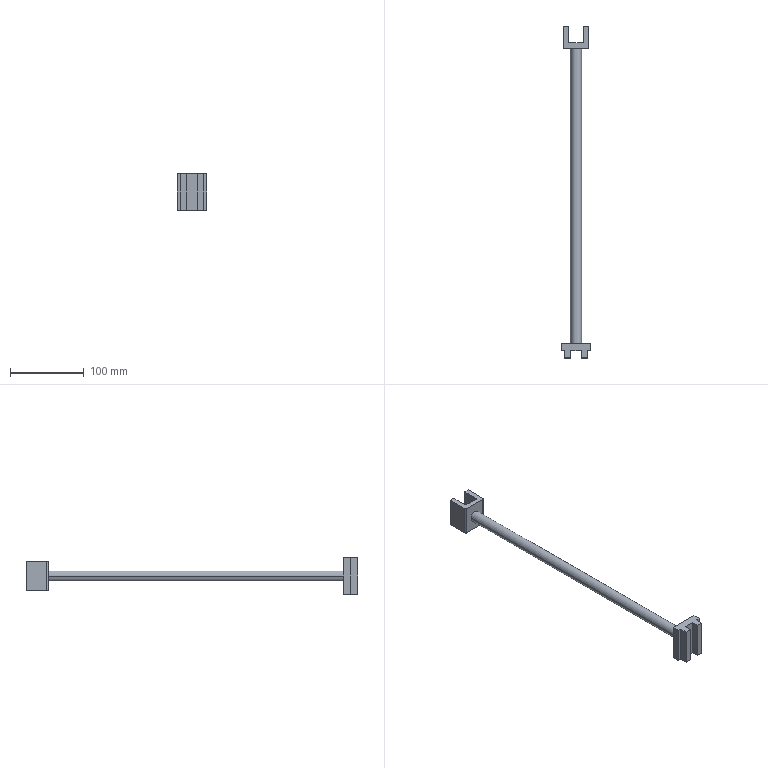Part | SolidWorks | features ICE 3, Extrusion 1, Fillet 1 | 1 solid | 30 faces | box 40 x 450 x 50 mm | volume 121566 mm3 | plane 24 | cylinder 6 | commonest cylinder face diameters 4 x4 15 x2
STEP:
#1=CARTESIAN_POINT('',(7.5,-415.,0.));
#2=VERTEX_POINT('',#1);
#3=CARTESIAN_POINT('',(-7.5,-415.,0.));
#4=VERTEX_POINT('',#3);
#5=CARTESIAN_POINT('',(0.,-415.,0.));
#6=DIRECTION('',(0.,-1.,0.));
#7=DIRECTION('',(1.,0.,0.));
#8=AXIS2_PLACEMENT_3D('',#5,#6,#7);
#9=CIRCLE('',#8,7.5);
#10=EDGE_CURVE('',#2,#4,#9,.T.);
#11=ORIENTED_EDGE('',*,*,#10,.F.);
#12=CARTESIAN_POINT('',(7.5,-15.,0.));
#13=VERTEX_POINT('',#12);
#14=CARTESIAN_POINT('',(7.5,-415.,0.));
#15=DIRECTION('',(0.,1.,0.));
#16=VECTOR('',#15,1000.);
#17=LINE('',#14,#16);
#18=EDGE_CURVE('',#2,#13,#17,.T.);
#19=ORIENTED_EDGE('',*,*,#18,.T.);
#20=CARTESIAN_POINT('',(-7.5,-15.,0.));
#21=VERTEX_POINT('',#20);
#22=CARTESIAN_POINT('',(0.,-15.,0.));
#23=DIRECTION('',(0.,-1.,0.));
#24=DIRECTION('',(-1.,0.,0.));
#25=AXIS2_PLACEMENT_3D('',#22,#23,#24);
#26=CIRCLE('',#25,7.5);
#27=EDGE_CURVE('',#13,#21,#26,.T.);
#28=ORIENTED_EDGE('',*,*,#27,.T.);
#29=CARTESIAN_POINT('',(-7.5,-415.,0.));
#30=DIRECTION('',(0.,1.,0.));
#31=VECTOR('',#30,1000.);
#32=LINE('',#29,#31);
#33=EDGE_CURVE('',#4,#21,#32,.T.);
#34=ORIENTED_EDGE('',*,*,#33,.F.);
#35=EDGE_LOOP('',(#11,#19,#28,#34));
#36=FACE_OUTER_BOUND('',#35,.T.);
#37=CARTESIAN_POINT('',(0.,-415.,0.));
#38=DIRECTION('',(0.,1.,0.));
#39=DIRECTION('',(-1.,0.,0.));
#40=AXIS2_PLACEMENT_3D('',#37,#38,#39);
#41=CYLINDRICAL_SURFACE('',#40,7.5);
#42=ADVANCED_FACE('',(#36),#41,.T.);
#43=CARTESIAN_POINT('',(20.,-425.,25.));
#44=VERTEX_POINT('',#43);
#45=CARTESIAN_POINT('',(15.1,-425.,25.));
#46=VERTEX_POINT('',#45);
#47=CARTESIAN_POINT('',(-20.,-425.,25.));
#48=DIRECTION('',(-1.,0.,0.));
#49=VECTOR('',#48,1000.);
#50=LINE('',#47,#49);
#51=EDGE_CURVE('',#44,#46,#50,.T.);
#52=ORIENTED_EDGE('',*,*,#51,.T.);
#53=CARTESIAN_POINT('',(15.1,-425.,-25.));
#54=VERTEX_POINT('',#53);
#55=CARTESIAN_POINT('',(15.1,-425.,25.));
#56=DIRECTION('',(0.,0.,1.));
#57=VECTOR('',#56,1000.);
#58=LINE('',#55,#57);
#59=EDGE_CURVE('',#54,#46,#58,.T.);
#60=ORIENTED_EDGE('',*,*,#59,.F.);
#61=CARTESIAN_POINT('',(20.,-425.,-25.));
#62=VERTEX_POINT('',#61);
#63=CARTESIAN_POINT('',(-20.,-425.,-25.));
#64=DIRECTION('',(1.,0.,0.));
#65=VECTOR('',#64,1000.);
#66=LINE('',#63,#65);
#67=EDGE_CURVE('',#54,#62,#66,.T.);
#68=ORIENTED_EDGE('',*,*,#67,.T.);
#69=CARTESIAN_POINT('',(20.,-425.,25.));
#70=DIRECTION('',(0.,0.,1.));
#71=VECTOR('',#70,1000.);
#72=LINE('',#69,#71);
#73=EDGE_CURVE('',#62,#44,#72,.T.);
#74=ORIENTED_EDGE('',*,*,#73,.T.);
#75=EDGE_LOOP('',(#52,#60,#68,#74));
#76=FACE_OUTER_BOUND('',#75,.T.);
#77=CARTESIAN_POINT('',(0.,-425.,0.));
#78=DIRECTION('',(0.,-1.,0.));
#79=DIRECTION('',(0.,0.,-1.));
#80=AXIS2_PLACEMENT_3D('',#77,#78,#79);
#81=PLANE('',#80);
#82=ADVANCED_FACE('',(#76),#81,.T.);
#83=CARTESIAN_POINT('',(-6.9,-425.,-25.));
#84=VERTEX_POINT('',#83);
#85=CARTESIAN_POINT('',(6.9,-425.,-25.));
#86=VERTEX_POINT('',#85);
#87=CARTESIAN_POINT('',(-20.,-425.,-25.));
#88=DIRECTION('',(1.,0.,0.));
#89=VECTOR('',#88,1000.);
#90=LINE('',#87,#89);
#91=EDGE_CURVE('',#84,#86,#90,.T.);
#92=ORIENTED_EDGE('',*,*,#91,.T.);
#93=CARTESIAN_POINT('',(6.9,-425.,25.));
#94=VERTEX_POINT('',#93);
#95=CARTESIAN_POINT('',(6.9,-425.,25.));
#96=DIRECTION('',(0.,0.,-1.));
#97=VECTOR('',#96,1000.);
#98=LINE('',#95,#97);
#99=EDGE_CURVE('',#94,#86,#98,.T.);
#100=ORIENTED_EDGE('',*,*,#99,.F.);
#101=CARTESIAN_POINT('',(-6.9,-425.,25.));
#102=VERTEX_POINT('',#101);
#103=CARTESIAN_POINT('',(-20.,-425.,25.));
#104=DIRECTION('',(-1.,0.,0.));
#105=VECTOR('',#104,1000.);
#106=LINE('',#103,#105);
#107=EDGE_CURVE('',#94,#102,#106,.T.);
#108=ORIENTED_EDGE('',*,*,#107,.T.);
#109=CARTESIAN_POINT('',(-6.9,-425.,25.));
#110=DIRECTION('',(0.,0.,1.));
#111=VECTOR('',#110,1000.);
#112=LINE('',#109,#111);
#113=EDGE_CURVE('',#84,#102,#112,.T.);
#114=ORIENTED_EDGE('',*,*,#113,.F.);
#115=EDGE_LOOP('',(#92,#100,#108,#114));
#116=FACE_OUTER_BOUND('',#115,.T.);
#117=CARTESIAN_POINT('',(0.,-425.,0.));
#118=DIRECTION('',(0.,-1.,0.));
#119=DIRECTION('',(0.,0.,-1.));
#120=AXIS2_PLACEMENT_3D('',#117,#118,#119);
#121=PLANE('',#120);
#122=ADVANCED_FACE('',(#116),#121,.T.);
#123=CARTESIAN_POINT('',(17.5,-13.,20.));
#124=VERTEX_POINT('',#123);
#125=CARTESIAN_POINT('',(17.5,15.,20.));
#126=VERTEX_POINT('',#125);
#127=CARTESIAN_POINT('',(17.5,15.,20.));
#128=DIRECTION('',(0.,1.,0.));
#129=VECTOR('',#128,1000.);
#130=LINE('',#127,#129);
#131=EDGE_CURVE('',#124,#126,#130,.T.);
#132=ORIENTED_EDGE('',*,*,#131,.F.);
#133=CARTESIAN_POINT('',(17.5,-13.,-20.));
#134=VERTEX_POINT('',#133);
#135=CARTESIAN_POINT('',(17.5,-13.,20.));
#136=DIRECTION('',(0.,0.,-1.));
#137=VECTOR('',#136,1000.);
#138=LINE('',#135,#137);
#139=EDGE_CURVE('',#124,#134,#138,.T.);
#140=ORIENTED_EDGE('',*,*,#139,.T.);
#141=CARTESIAN_POINT('',(17.5,15.,-20.));
#142=VERTEX_POINT('',#141);
#143=CARTESIAN_POINT('',(17.5,15.,-20.));
#144=DIRECTION('',(0.,1.,0.));
#145=VECTOR('',#144,1000.);
#146=LINE('',#143,#145);
#147=EDGE_CURVE('',#134,#142,#146,.T.);
#148=ORIENTED_EDGE('',*,*,#147,.T.);
#149=CARTESIAN_POINT('',(17.5,15.,20.));
#150=DIRECTION('',(0.,0.,-1.));
#151=VECTOR('',#150,1000.);
#152=LINE('',#149,#151);
#153=EDGE_CURVE('',#126,#142,#152,.T.);
#154=ORIENTED_EDGE('',*,*,#153,.F.);
#155=EDGE_LOOP('',(#132,#140,#148,#154));
#156=FACE_OUTER_BOUND('',#155,.T.);
#157=CARTESIAN_POINT('',(17.5,15.,20.));
#158=DIRECTION('',(-1.,0.,0.));
#159=DIRECTION('',(0.,-1.,0.));
#160=AXIS2_PLACEMENT_3D('',#157,#158,#159);
#161=PLANE('',#160);
#162=ADVANCED_FACE('',(#156),#161,.F.);
#163=CARTESIAN_POINT('',(10.5,15.,-20.));
#164=VERTEX_POINT('',#163);
#165=CARTESIAN_POINT('',(10.5,15.,-20.));
#166=DIRECTION('',(-1.,0.,0.));
#167=VECTOR('',#166,1000.);
#168=LINE('',#165,#167);
#169=EDGE_CURVE('',#142,#164,#168,.T.);
#170=ORIENTED_EDGE('',*,*,#169,.T.);
#171=CARTESIAN_POINT('',(10.5,15.,20.));
#172=VERTEX_POINT('',#171);
#173=CARTESIAN_POINT('',(10.5,15.,20.));
#174=DIRECTION('',(0.,0.,-1.));
#175=VECTOR('',#174,1000.);
#176=LINE('',#173,#175);
#177=EDGE_CURVE('',#172,#164,#176,.T.);
#178=ORIENTED_EDGE('',*,*,#177,.F.);
#179=CARTESIAN_POINT('',(10.5,15.,20.));
#180=DIRECTION('',(-1.,0.,0.));
#181=VECTOR('',#180,1000.);
#182=LINE('',#179,#181);
#183=EDGE_CURVE('',#126,#172,#182,.T.);
#184=ORIENTED_EDGE('',*,*,#183,.F.);
#185=ORIENTED_EDGE('',*,*,#153,.T.);
#186=EDGE_LOOP('',(#170,#178,#184,#185));
#187=FACE_OUTER_BOUND('',#186,.T.);
#188=CARTESIAN_POINT('',(10.5,15.,20.));
#189=DIRECTION('',(0.,-1.,0.));
#190=DIRECTION('',(0.,0.,-1.));
#191=AXIS2_PLACEMENT_3D('',#188,#189,#190);
#192=PLANE('',#191);
#193=ADVANCED_FACE('',(#187),#192,.F.);
#194=CARTESIAN_POINT('',(10.5,-6.,-20.));
#195=VERTEX_POINT('',#194);
#196=CARTESIAN_POINT('',(10.5,8.,-20.));
#197=DIRECTION('',(0.,-1.,0.));
#198=VECTOR('',#197,1000.);
#199=LINE('',#196,#198);
#200=EDGE_CURVE('',#164,#195,#199,.T.);
#201=ORIENTED_EDGE('',*,*,#200,.T.);
#202=CARTESIAN_POINT('',(10.5,-6.,20.));
#203=VERTEX_POINT('',#202);
#204=CARTESIAN_POINT('',(10.5,-6.,20.));
#205=DIRECTION('',(0.,0.,1.));
#206=VECTOR('',#205,1000.);
#207=LINE('',#204,#206);
#208=EDGE_CURVE('',#195,#203,#207,.T.);
#209=ORIENTED_EDGE('',*,*,#208,.T.);
#210=CARTESIAN_POINT('',(10.5,8.,20.));
#211=DIRECTION('',(0.,-1.,0.));
#212=VECTOR('',#211,1000.);
#213=LINE('',#210,#212);
#214=EDGE_CURVE('',#172,#203,#213,.T.);
#215=ORIENTED_EDGE('',*,*,#214,.F.);
#216=ORIENTED_EDGE('',*,*,#177,.T.);
#217=EDGE_LOOP('',(#201,#209,#215,#216));
#218=FACE_OUTER_BOUND('',#217,.T.);
#219=CARTESIAN_POINT('',(10.5,8.,20.));
#220=DIRECTION('',(1.,0.,0.));
#221=DIRECTION('',(0.,1.,0.));
#222=AXIS2_PLACEMENT_3D('',#219,#220,#221);
#223=PLANE('',#222);
#224=ADVANCED_FACE('',(#218),#223,.F.);
#225=CARTESIAN_POINT('',(8.5,-8.,20.));
#226=VERTEX_POINT('',#225);
#227=CARTESIAN_POINT('',(-8.5,-8.,20.));
#228=VERTEX_POINT('',#227);
#229=CARTESIAN_POINT('',(-10.5,-8.,20.));
#230=DIRECTION('',(-1.,0.,0.));
#231=VECTOR('',#230,1000.);
#232=LINE('',#229,#231);
#233=EDGE_CURVE('',#226,#228,#232,.T.);
#234=ORIENTED_EDGE('',*,*,#233,.F.);
#235=CARTESIAN_POINT('',(8.5,-8.,-20.));
#236=VERTEX_POINT('',#235);
#237=CARTESIAN_POINT('',(8.5,-8.,-20.));
#238=DIRECTION('',(0.,0.,-1.));
#239=VECTOR('',#238,1000.);
#240=LINE('',#237,#239);
#241=EDGE_CURVE('',#226,#236,#240,.T.);
#242=ORIENTED_EDGE('',*,*,#241,.T.);
#243=CARTESIAN_POINT('',(-8.5,-8.,-20.));
#244=VERTEX_POINT('',#243);
#245=CARTESIAN_POINT('',(-10.5,-8.,-20.));
#246=DIRECTION('',(-1.,0.,0.));
#247=VECTOR('',#246,1000.);
#248=LINE('',#245,#247);
#249=EDGE_CURVE('',#236,#244,#248,.T.);
#250=ORIENTED_EDGE('',*,*,#249,.T.);
#251=CARTESIAN_POINT('',(-8.5,-8.,20.));
#252=DIRECTION('',(0.,0.,1.));
#253=VECTOR('',#252,1000.);
#254=LINE('',#251,#253);
#255=EDGE_CURVE('',#244,#228,#254,.T.);
#256=ORIENTED_EDGE('',*,*,#255,.T.);
#257=EDGE_LOOP('',(#234,#242,#250,#256));
#258=FACE_OUTER_BOUND('',#257,.T.);
#259=CARTESIAN_POINT('',(-10.5,-8.,20.));
#260=DIRECTION('',(0.,-1.,0.));
#261=DIRECTION('',(0.,0.,-1.));
#262=AXIS2_PLACEMENT_3D('',#259,#260,#261);
#263=PLANE('',#262);
#264=ADVANCED_FACE('',(#258),#263,.F.);
#265=CARTESIAN_POINT('',(-10.5,-6.,20.));
#266=VERTEX_POINT('',#265);
#267=CARTESIAN_POINT('',(-10.5,15.,20.));
#268=VERTEX_POINT('',#267);
#269=CARTESIAN_POINT('',(-10.5,8.,20.));
#270=DIRECTION('',(0.,1.,0.));
#271=VECTOR('',#270,1000.);
#272=LINE('',#269,#271);
#273=EDGE_CURVE('',#266,#268,#272,.T.);
#274=ORIENTED_EDGE('',*,*,#273,.F.);
#275=CARTESIAN_POINT('',(-10.5,-6.,-20.));
#276=VERTEX_POINT('',#275);
#277=CARTESIAN_POINT('',(-10.5,-6.,-20.));
#278=DIRECTION('',(0.,0.,-1.));
#279=VECTOR('',#278,1000.);
#280=LINE('',#277,#279);
#281=EDGE_CURVE('',#266,#276,#280,.T.);
#282=ORIENTED_EDGE('',*,*,#281,.T.);
#283=CARTESIAN_POINT('',(-10.5,15.,-20.));
#284=VERTEX_POINT('',#283);
#285=CARTESIAN_POINT('',(-10.5,8.,-20.));
#286=DIRECTION('',(0.,1.,0.));
#287=VECTOR('',#286,1000.);
#288=LINE('',#285,#287);
#289=EDGE_CURVE('',#276,#284,#288,.T.);
#290=ORIENTED_EDGE('',*,*,#289,.T.);
#291=CARTESIAN_POINT('',(-10.5,15.,20.));
#292=DIRECTION('',(0.,0.,-1.));
#293=VECTOR('',#292,1000.);
#294=LINE('',#291,#293);
#295=EDGE_CURVE('',#268,#284,#294,.T.);
#296=ORIENTED_EDGE('',*,*,#295,.F.);
#297=EDGE_LOOP('',(#274,#282,#290,#296));
#298=FACE_OUTER_BOUND('',#297,.T.);
#299=CARTESIAN_POINT('',(-10.5,8.,20.));
#300=DIRECTION('',(-1.,0.,0.));
#301=DIRECTION('',(0.,-1.,0.));
#302=AXIS2_PLACEMENT_3D('',#299,#300,#301);
#303=PLANE('',#302);
#304=ADVANCED_FACE('',(#298),#303,.F.);
#305=CARTESIAN_POINT('',(-17.5,15.,-20.));
#306=VERTEX_POINT('',#305);
#307=CARTESIAN_POINT('',(-17.5,15.,-20.));
#308=DIRECTION('',(-1.,0.,0.));
#309=VECTOR('',#308,1000.);
#310=LINE('',#307,#309);
#311=EDGE_CURVE('',#284,#306,#310,.T.);
#312=ORIENTED_EDGE('',*,*,#311,.T.);
#313=CARTESIAN_POINT('',(-17.5,15.,20.));
#314=VERTEX_POINT('',#313);
#315=CARTESIAN_POINT('',(-17.5,15.,20.));
#316=DIRECTION('',(0.,0.,-1.));
#317=VECTOR('',#316,1000.);
#318=LINE('',#315,#317);
#319=EDGE_CURVE('',#314,#306,#318,.T.);
#320=ORIENTED_EDGE('',*,*,#319,.F.);
#321=CARTESIAN_POINT('',(-17.5,15.,20.));
#322=DIRECTION('',(-1.,0.,0.));
#323=VECTOR('',#322,1000.);
#324=LINE('',#321,#323);
#325=EDGE_CURVE('',#268,#314,#324,.T.);
#326=ORIENTED_EDGE('',*,*,#325,.F.);
#327=ORIENTED_EDGE('',*,*,#295,.T.);
#328=EDGE_LOOP('',(#312,#320,#326,#327));
#329=FACE_OUTER_BOUND('',#328,.T.);
#330=CARTESIAN_POINT('',(-17.5,15.,20.));
#331=DIRECTION('',(0.,-1.,0.));
#332=DIRECTION('',(0.,0.,-1.));
#333=AXIS2_PLACEMENT_3D('',#330,#331,#332);
#334=PLANE('',#333);
#335=ADVANCED_FACE('',(#329),#334,.F.);
#336=CARTESIAN_POINT('',(-17.5,-13.,-20.));
#337=VERTEX_POINT('',#336);
#338=CARTESIAN_POINT('',(-17.5,15.,-20.));
#339=DIRECTION('',(0.,-1.,0.));
#340=VECTOR('',#339,1000.);
#341=LINE('',#338,#340);
#342=EDGE_CURVE('',#306,#337,#341,.T.);
#343=ORIENTED_EDGE('',*,*,#342,.T.);
#344=CARTESIAN_POINT('',(-17.5,-13.,20.));
#345=VERTEX_POINT('',#344);
#346=CARTESIAN_POINT('',(-17.5,-13.,20.));
#347=DIRECTION('',(0.,0.,1.));
#348=VECTOR('',#347,1000.);
#349=LINE('',#346,#348);
#350=EDGE_CURVE('',#337,#345,#349,.T.);
#351=ORIENTED_EDGE('',*,*,#350,.T.);
#352=CARTESIAN_POINT('',(-17.5,15.,20.));
#353=DIRECTION('',(0.,-1.,0.));
#354=VECTOR('',#353,1000.);
#355=LINE('',#352,#354);
#356=EDGE_CURVE('',#314,#345,#355,.T.);
#357=ORIENTED_EDGE('',*,*,#356,.F.);
#358=ORIENTED_EDGE('',*,*,#319,.T.);
#359=EDGE_LOOP('',(#343,#351,#357,#358));
#360=FACE_OUTER_BOUND('',#359,.T.);
#361=CARTESIAN_POINT('',(-17.5,15.,20.));
#362=DIRECTION('',(1.,0.,0.));
#363=DIRECTION('',(0.,1.,0.));
#364=AXIS2_PLACEMENT_3D('',#361,#362,#363);
#365=PLANE('',#364);
#366=ADVANCED_FACE('',(#360),#365,.F.);
#367=CARTESIAN_POINT('',(0.,-15.,0.));
#368=DIRECTION('',(0.,-1.,0.));
#369=DIRECTION('',(-1.,0.,0.));
#370=AXIS2_PLACEMENT_3D('',#367,#368,#369);
#371=CIRCLE('',#370,7.5);
#372=EDGE_CURVE('',#21,#13,#371,.T.);
#373=ORIENTED_EDGE('',*,*,#372,.F.);
#374=ORIENTED_EDGE('',*,*,#27,.F.);
#375=EDGE_LOOP('',(#373,#374));
#376=FACE_BOUND('',#375,.T.);
#377=CARTESIAN_POINT('',(-15.5,-15.,-20.));
#378=VERTEX_POINT('',#377);
#379=CARTESIAN_POINT('',(15.5,-15.,-20.));
#380=VERTEX_POINT('',#379);
#381=CARTESIAN_POINT('',(-17.5,-15.,-20.));
#382=DIRECTION('',(1.,0.,0.));
#383=VECTOR('',#382,1000.);
#384=LINE('',#381,#383);
#385=EDGE_CURVE('',#378,#380,#384,.T.);
#386=ORIENTED_EDGE('',*,*,#385,.T.);
#387=CARTESIAN_POINT('',(15.5,-15.,20.));
#388=VERTEX_POINT('',#387);
#389=CARTESIAN_POINT('',(15.5,-15.,20.));
#390=DIRECTION('',(0.,0.,1.));
#391=VECTOR('',#390,1000.);
#392=LINE('',#389,#391);
#393=EDGE_CURVE('',#380,#388,#392,.T.);
#394=ORIENTED_EDGE('',*,*,#393,.T.);
#395=CARTESIAN_POINT('',(-15.5,-15.,20.));
#396=VERTEX_POINT('',#395);
#397=CARTESIAN_POINT('',(-17.5,-15.,20.));
#398=DIRECTION('',(1.,0.,0.));
#399=VECTOR('',#398,1000.);
#400=LINE('',#397,#399);
#401=EDGE_CURVE('',#396,#388,#400,.T.);
#402=ORIENTED_EDGE('',*,*,#401,.F.);
#403=CARTESIAN_POINT('',(-15.5,-15.,20.));
#404=DIRECTION('',(0.,0.,-1.));
#405=VECTOR('',#404,1000.);
#406=LINE('',#403,#405);
#407=EDGE_CURVE('',#396,#378,#406,.T.);
#408=ORIENTED_EDGE('',*,*,#407,.T.);
#409=EDGE_LOOP('',(#386,#394,#402,#408));
#410=FACE_OUTER_BOUND('',#409,.T.);
#411=CARTESIAN_POINT('',(-17.5,-15.,20.));
#412=DIRECTION('',(0.,1.,0.));
#413=DIRECTION('',(-1.,0.,0.));
#414=AXIS2_PLACEMENT_3D('',#411,#412,#413);
#415=PLANE('',#414);
#416=ADVANCED_FACE('',(#376,#410),#415,.F.);
#417=ORIENTED_EDGE('',*,*,#401,.T.);
#418=CARTESIAN_POINT('',(15.5,-13.,20.));
#419=DIRECTION('',(0.,0.,1.));
#420=DIRECTION('',(1.,0.,0.));
#421=AXIS2_PLACEMENT_3D('',#418,#419,#420);
#422=CIRCLE('',#421,2.);
#423=EDGE_CURVE('',#388,#124,#422,.T.);
#424=ORIENTED_EDGE('',*,*,#423,.T.);
#425=ORIENTED_EDGE('',*,*,#131,.T.);
#426=ORIENTED_EDGE('',*,*,#183,.T.);
#427=ORIENTED_EDGE('',*,*,#214,.T.);
#428=CARTESIAN_POINT('',(8.5,-6.,20.));
#429=DIRECTION('',(0.,0.,-1.));
#430=DIRECTION('',(1.,0.,0.));
#431=AXIS2_PLACEMENT_3D('',#428,#429,#430);
#432=CIRCLE('',#431,2.);
#433=EDGE_CURVE('',#203,#226,#432,.T.);
#434=ORIENTED_EDGE('',*,*,#433,.T.);
#435=ORIENTED_EDGE('',*,*,#233,.T.);
#436=CARTESIAN_POINT('',(-8.5,-6.,20.));
#437=DIRECTION('',(0.,0.,-1.));
#438=DIRECTION('',(1.,0.,0.));
#439=AXIS2_PLACEMENT_3D('',#436,#437,#438);
#440=CIRCLE('',#439,2.);
#441=EDGE_CURVE('',#228,#266,#440,.T.);
#442=ORIENTED_EDGE('',*,*,#441,.T.);
#443=ORIENTED_EDGE('',*,*,#273,.T.);
#444=ORIENTED_EDGE('',*,*,#325,.T.);
#445=ORIENTED_EDGE('',*,*,#356,.T.);
#446=CARTESIAN_POINT('',(-15.5,-13.,20.));
#447=DIRECTION('',(0.,0.,1.));
#448=DIRECTION('',(1.,0.,0.));
#449=AXIS2_PLACEMENT_3D('',#446,#447,#448);
#450=CIRCLE('',#449,2.);
#451=EDGE_CURVE('',#345,#396,#450,.T.);
#452=ORIENTED_EDGE('',*,*,#451,.T.);
#453=EDGE_LOOP('',(#417,#424,#425,#426,#427,#434,#435,#442,#443,#444,#445,#452));
#454=FACE_OUTER_BOUND('',#453,.T.);
#455=CARTESIAN_POINT('',(0.,0.,20.));
#456=DIRECTION('',(0.,0.,1.));
#457=DIRECTION('',(1.,0.,0.));
#458=AXIS2_PLACEMENT_3D('',#455,#456,#457);
#459=PLANE('',#458);
#460=ADVANCED_FACE('',(#454),#459,.T.);
#461=ORIENTED_EDGE('',*,*,#147,.F.);
#462=CARTESIAN_POINT('',(15.5,-13.,-20.));
#463=DIRECTION('',(0.,0.,-1.));
#464=DIRECTION('',(1.,0.,0.));
#465=AXIS2_PLACEMENT_3D('',#462,#463,#464);
#466=CIRCLE('',#465,2.);
#467=EDGE_CURVE('',#134,#380,#466,.T.);
#468=ORIENTED_EDGE('',*,*,#467,.T.);
#469=ORIENTED_EDGE('',*,*,#385,.F.);
#470=CARTESIAN_POINT('',(-15.5,-13.,-20.));
#471=DIRECTION('',(0.,0.,-1.));
#472=DIRECTION('',(1.,0.,0.));
#473=AXIS2_PLACEMENT_3D('',#470,#471,#472);
#474=CIRCLE('',#473,2.);
#475=EDGE_CURVE('',#378,#337,#474,.T.);
#476=ORIENTED_EDGE('',*,*,#475,.T.);
#477=ORIENTED_EDGE('',*,*,#342,.F.);
#478=ORIENTED_EDGE('',*,*,#311,.F.);
#479=ORIENTED_EDGE('',*,*,#289,.F.);
#480=CARTESIAN_POINT('',(-8.5,-6.,-20.));
#481=DIRECTION('',(0.,0.,1.));
#482=DIRECTION('',(1.,0.,0.));
#483=AXIS2_PLACEMENT_3D('',#480,#481,#482);
#484=CIRCLE('',#483,2.);
#485=EDGE_CURVE('',#276,#244,#484,.T.);
#486=ORIENTED_EDGE('',*,*,#485,.T.);
#487=ORIENTED_EDGE('',*,*,#249,.F.);
#488=CARTESIAN_POINT('',(8.5,-6.,-20.));
#489=DIRECTION('',(0.,0.,1.));
#490=DIRECTION('',(1.,0.,0.));
#491=AXIS2_PLACEMENT_3D('',#488,#489,#490);
#492=CIRCLE('',#491,2.);
#493=EDGE_CURVE('',#236,#195,#492,.T.);
#494=ORIENTED_EDGE('',*,*,#493,.T.);
#495=ORIENTED_EDGE('',*,*,#200,.F.);
#496=ORIENTED_EDGE('',*,*,#169,.F.);
#497=EDGE_LOOP('',(#461,#468,#469,#476,#477,#478,#479,#486,#487,#494,#495,#496));
#498=FACE_OUTER_BOUND('',#497,.T.);
#499=CARTESIAN_POINT('',(0.,0.,-20.));
#500=DIRECTION('',(0.,0.,1.));
#501=DIRECTION('',(1.,0.,0.));
#502=AXIS2_PLACEMENT_3D('',#499,#500,#501);
#503=PLANE('',#502);
#504=ADVANCED_FACE('',(#498),#503,.F.);
#505=ORIENTED_EDGE('',*,*,#423,.F.);
#506=ORIENTED_EDGE('',*,*,#393,.F.);
#507=ORIENTED_EDGE('',*,*,#467,.F.);
#508=ORIENTED_EDGE('',*,*,#139,.F.);
#509=EDGE_LOOP('',(#505,#506,#507,#508));
#510=FACE_OUTER_BOUND('',#509,.T.);
#511=CARTESIAN_POINT('',(15.5,-13.,20.));
#512=DIRECTION('',(0.,0.,-1.));
#513=DIRECTION('',(-1.,0.,0.));
#514=AXIS2_PLACEMENT_3D('',#511,#512,#513);
#515=CYLINDRICAL_SURFACE('',#514,2.);
#516=ADVANCED_FACE('',(#510),#515,.T.);
#517=ORIENTED_EDGE('',*,*,#451,.F.);
#518=ORIENTED_EDGE('',*,*,#350,.F.);
#519=ORIENTED_EDGE('',*,*,#475,.F.);
#520=ORIENTED_EDGE('',*,*,#407,.F.);
#521=EDGE_LOOP('',(#517,#518,#519,#520));
#522=FACE_OUTER_BOUND('',#521,.T.);
#523=CARTESIAN_POINT('',(-15.5,-13.,20.));
#524=DIRECTION('',(0.,0.,-1.));
#525=DIRECTION('',(-1.,0.,0.));
#526=AXIS2_PLACEMENT_3D('',#523,#524,#525);
#527=CYLINDRICAL_SURFACE('',#526,2.);
#528=ADVANCED_FACE('',(#522),#527,.T.);
#529=ORIENTED_EDGE('',*,*,#433,.F.);
#530=ORIENTED_EDGE('',*,*,#208,.F.);
#531=ORIENTED_EDGE('',*,*,#493,.F.);
#532=ORIENTED_EDGE('',*,*,#241,.F.);
#533=EDGE_LOOP('',(#529,#530,#531,#532));
#534=FACE_OUTER_BOUND('',#533,.T.);
#535=CARTESIAN_POINT('',(8.5,-6.,20.));
#536=DIRECTION('',(0.,0.,1.));
#537=DIRECTION('',(1.,0.,0.));
#538=AXIS2_PLACEMENT_3D('',#535,#536,#537);
#539=CYLINDRICAL_SURFACE('',#538,2.);
#540=ADVANCED_FACE('',(#534),#539,.F.);
#541=ORIENTED_EDGE('',*,*,#441,.F.);
#542=ORIENTED_EDGE('',*,*,#255,.F.);
#543=ORIENTED_EDGE('',*,*,#485,.F.);
#544=ORIENTED_EDGE('',*,*,#281,.F.);
#545=EDGE_LOOP('',(#541,#542,#543,#544));
#546=FACE_OUTER_BOUND('',#545,.T.);
#547=CARTESIAN_POINT('',(-8.5,-6.,20.));
#548=DIRECTION('',(0.,0.,1.));
#549=DIRECTION('',(1.,0.,0.));
#550=AXIS2_PLACEMENT_3D('',#547,#548,#549);
#551=CYLINDRICAL_SURFACE('',#550,2.);
#552=ADVANCED_FACE('',(#546),#551,.F.);
#553=ORIENTED_EDGE('',*,*,#18,.F.);
#554=CARTESIAN_POINT('',(0.,-415.,0.));
#555=DIRECTION('',(0.,-1.,0.));
#556=DIRECTION('',(1.,0.,0.));
#557=AXIS2_PLACEMENT_3D('',#554,#555,#556);
#558=CIRCLE('',#557,7.5);
#559=EDGE_CURVE('',#4,#2,#558,.T.);
#560=ORIENTED_EDGE('',*,*,#559,.F.);
#561=ORIENTED_EDGE('',*,*,#33,.T.);
#562=ORIENTED_EDGE('',*,*,#372,.T.);
#563=EDGE_LOOP('',(#553,#560,#561,#562));
#564=FACE_OUTER_BOUND('',#563,.T.);
#565=CARTESIAN_POINT('',(0.,-415.,0.));
#566=DIRECTION('',(0.,1.,0.));
#567=DIRECTION('',(-1.,0.,0.));
#568=AXIS2_PLACEMENT_3D('',#565,#566,#567);
#569=CYLINDRICAL_SURFACE('',#568,7.5);
#570=ADVANCED_FACE('',(#564),#569,.T.);
#571=CARTESIAN_POINT('',(20.,-415.,-25.));
#572=VERTEX_POINT('',#571);
#573=CARTESIAN_POINT('',(20.,-415.,25.));
#574=VERTEX_POINT('',#573);
#575=CARTESIAN_POINT('',(20.,-415.,25.));
#576=DIRECTION('',(0.,0.,1.));
#577=VECTOR('',#576,1000.);
#578=LINE('',#575,#577);
#579=EDGE_CURVE('',#572,#574,#578,.T.);
#580=ORIENTED_EDGE('',*,*,#579,.T.);
#581=CARTESIAN_POINT('',(20.,-425.,25.));
#582=DIRECTION('',(0.,1.,0.));
#583=VECTOR('',#582,1000.);
#584=LINE('',#581,#583);
#585=EDGE_CURVE('',#44,#574,#584,.T.);
#586=ORIENTED_EDGE('',*,*,#585,.F.);
#587=ORIENTED_EDGE('',*,*,#73,.F.);
#588=CARTESIAN_POINT('',(20.,-425.,-25.));
#589=DIRECTION('',(0.,1.,0.));
#590=VECTOR('',#589,1000.);
#591=LINE('',#588,#590);
#592=EDGE_CURVE('',#62,#572,#591,.T.);
#593=ORIENTED_EDGE('',*,*,#592,.T.);
#594=EDGE_LOOP('',(#580,#586,#587,#593));
#595=FACE_OUTER_BOUND('',#594,.T.);
#596=CARTESIAN_POINT('',(20.,-425.,25.));
#597=DIRECTION('',(-1.,0.,0.));
#598=DIRECTION('',(0.,0.,1.));
#599=AXIS2_PLACEMENT_3D('',#596,#597,#598);
#600=PLANE('',#599);
#601=ADVANCED_FACE('',(#595),#600,.F.);
#602=CARTESIAN_POINT('',(-20.,-415.,25.));
#603=VERTEX_POINT('',#602);
#604=CARTESIAN_POINT('',(-20.,-415.,25.));
#605=DIRECTION('',(-1.,0.,0.));
#606=VECTOR('',#605,1000.);
#607=LINE('',#604,#606);
#608=EDGE_CURVE('',#574,#603,#607,.T.);
#609=ORIENTED_EDGE('',*,*,#608,.T.);
#610=CARTESIAN_POINT('',(-20.,-425.,25.));
#611=VERTEX_POINT('',#610);
#612=CARTESIAN_POINT('',(-20.,-425.,25.));
#613=DIRECTION('',(0.,1.,0.));
#614=VECTOR('',#613,1000.);
#615=LINE('',#612,#614);
#616=EDGE_CURVE('',#611,#603,#615,.T.);
#617=ORIENTED_EDGE('',*,*,#616,.F.);
#618=CARTESIAN_POINT('',(-15.1,-425.,25.));
#619=VERTEX_POINT('',#618);
#620=CARTESIAN_POINT('',(-20.,-425.,25.));
#621=DIRECTION('',(-1.,0.,0.));
#622=VECTOR('',#621,1000.);
#623=LINE('',#620,#622);
#624=EDGE_CURVE('',#619,#611,#623,.T.);
#625=ORIENTED_EDGE('',*,*,#624,.F.);
#626=CARTESIAN_POINT('',(-15.1,-435.,25.));
#627=VERTEX_POINT('',#626);
#628=CARTESIAN_POINT('',(-15.1,-435.,25.));
#629=DIRECTION('',(0.,1.,0.));
#630=VECTOR('',#629,1000.);
#631=LINE('',#628,#630);
#632=EDGE_CURVE('',#627,#619,#631,.T.);
#633=ORIENTED_EDGE('',*,*,#632,.F.);
#634=CARTESIAN_POINT('',(-6.9,-435.,25.));
#635=VERTEX_POINT('',#634);
#636=CARTESIAN_POINT('',(-15.1,-435.,25.));
#637=DIRECTION('',(-1.,0.,0.));
#638=VECTOR('',#637,1000.);
#639=LINE('',#636,#638);
#640=EDGE_CURVE('',#635,#627,#639,.T.);
#641=ORIENTED_EDGE('',*,*,#640,.F.);
#642=CARTESIAN_POINT('',(-6.9,-435.,25.));
#643=DIRECTION('',(0.,1.,0.));
#644=VECTOR('',#643,1000.);
#645=LINE('',#642,#644);
#646=EDGE_CURVE('',#635,#102,#645,.T.);
#647=ORIENTED_EDGE('',*,*,#646,.T.);
#648=ORIENTED_EDGE('',*,*,#107,.F.);
#649=CARTESIAN_POINT('',(6.9,-435.,25.));
#650=VERTEX_POINT('',#649);
#651=CARTESIAN_POINT('',(6.9,-435.,25.));
#652=DIRECTION('',(0.,1.,0.));
#653=VECTOR('',#652,1000.);
#654=LINE('',#651,#653);
#655=EDGE_CURVE('',#650,#94,#654,.T.);
#656=ORIENTED_EDGE('',*,*,#655,.F.);
#657=CARTESIAN_POINT('',(15.1,-435.,25.));
#658=VERTEX_POINT('',#657);
#659=CARTESIAN_POINT('',(15.1,-435.,25.));
#660=DIRECTION('',(-1.,0.,0.));
#661=VECTOR('',#660,1000.);
#662=LINE('',#659,#661);
#663=EDGE_CURVE('',#658,#650,#662,.T.);
#664=ORIENTED_EDGE('',*,*,#663,.F.);
#665=CARTESIAN_POINT('',(15.1,-435.,25.));
#666=DIRECTION('',(0.,1.,0.));
#667=VECTOR('',#666,1000.);
#668=LINE('',#665,#667);
#669=EDGE_CURVE('',#658,#46,#668,.T.);
#670=ORIENTED_EDGE('',*,*,#669,.T.);
#671=ORIENTED_EDGE('',*,*,#51,.F.);
#672=ORIENTED_EDGE('',*,*,#585,.T.);
#673=EDGE_LOOP('',(#609,#617,#625,#633,#641,#647,#648,#656,#664,#670,#671,#672));
#674=FACE_OUTER_BOUND('',#673,.T.);
#675=CARTESIAN_POINT('',(-20.,-425.,25.));
#676=DIRECTION('',(0.,0.,-1.));
#677=DIRECTION('',(-1.,0.,0.));
#678=AXIS2_PLACEMENT_3D('',#675,#676,#677);
#679=PLANE('',#678);
#680=ADVANCED_FACE('',(#674),#679,.F.);
#681=CARTESIAN_POINT('',(-20.,-415.,-25.));
#682=VERTEX_POINT('',#681);
#683=CARTESIAN_POINT('',(-20.,-415.,25.));
#684=DIRECTION('',(0.,0.,-1.));
#685=VECTOR('',#684,1000.);
#686=LINE('',#683,#685);
#687=EDGE_CURVE('',#603,#682,#686,.T.);
#688=ORIENTED_EDGE('',*,*,#687,.T.);
#689=CARTESIAN_POINT('',(-20.,-425.,-25.));
#690=VERTEX_POINT('',#689);
#691=CARTESIAN_POINT('',(-20.,-425.,-25.));
#692=DIRECTION('',(0.,1.,0.));
#693=VECTOR('',#692,1000.);
#694=LINE('',#691,#693);
#695=EDGE_CURVE('',#690,#682,#694,.T.);
#696=ORIENTED_EDGE('',*,*,#695,.F.);
#697=CARTESIAN_POINT('',(-20.,-425.,25.));
#698=DIRECTION('',(0.,0.,-1.));
#699=VECTOR('',#698,1000.);
#700=LINE('',#697,#699);
#701=EDGE_CURVE('',#611,#690,#700,.T.);
#702=ORIENTED_EDGE('',*,*,#701,.F.);
#703=ORIENTED_EDGE('',*,*,#616,.T.);
#704=EDGE_LOOP('',(#688,#696,#702,#703));
#705=FACE_OUTER_BOUND('',#704,.T.);
#706=CARTESIAN_POINT('',(-20.,-425.,25.));
#707=DIRECTION('',(1.,0.,0.));
#708=DIRECTION('',(0.,0.,-1.));
#709=AXIS2_PLACEMENT_3D('',#706,#707,#708);
#710=PLANE('',#709);
#711=ADVANCED_FACE('',(#705),#710,.F.);
#712=CARTESIAN_POINT('',(-20.,-415.,-25.));
#713=DIRECTION('',(1.,0.,0.));
#714=VECTOR('',#713,1000.);
#715=LINE('',#712,#714);
#716=EDGE_CURVE('',#682,#572,#715,.T.);
#717=ORIENTED_EDGE('',*,*,#716,.T.);
#718=ORIENTED_EDGE('',*,*,#592,.F.);
#719=ORIENTED_EDGE('',*,*,#67,.F.);
#720=CARTESIAN_POINT('',(15.1,-435.,-25.));
#721=VERTEX_POINT('',#720);
#722=CARTESIAN_POINT('',(15.1,-435.,-25.));
#723=DIRECTION('',(0.,1.,0.));
#724=VECTOR('',#723,1000.);
#725=LINE('',#722,#724);
#726=EDGE_CURVE('',#721,#54,#725,.T.);
#727=ORIENTED_EDGE('',*,*,#726,.F.);
#728=CARTESIAN_POINT('',(6.9,-435.,-25.));
#729=VERTEX_POINT('',#728);
#730=CARTESIAN_POINT('',(15.1,-435.,-25.));
#731=DIRECTION('',(1.,0.,0.));
#732=VECTOR('',#731,1000.);
#733=LINE('',#730,#732);
#734=EDGE_CURVE('',#729,#721,#733,.T.);
#735=ORIENTED_EDGE('',*,*,#734,.F.);
#736=CARTESIAN_POINT('',(6.9,-435.,-25.));
#737=DIRECTION('',(0.,1.,0.));
#738=VECTOR('',#737,1000.);
#739=LINE('',#736,#738);
#740=EDGE_CURVE('',#729,#86,#739,.T.);
#741=ORIENTED_EDGE('',*,*,#740,.T.);
#742=ORIENTED_EDGE('',*,*,#91,.F.);
#743=CARTESIAN_POINT('',(-6.9,-435.,-25.));
#744=VERTEX_POINT('',#743);
#745=CARTESIAN_POINT('',(-6.9,-435.,-25.));
#746=DIRECTION('',(0.,1.,0.));
#747=VECTOR('',#746,1000.);
#748=LINE('',#745,#747);
#749=EDGE_CURVE('',#744,#84,#748,.T.);
#750=ORIENTED_EDGE('',*,*,#749,.F.);
#751=CARTESIAN_POINT('',(-15.1,-435.,-25.));
#752=VERTEX_POINT('',#751);
#753=CARTESIAN_POINT('',(-15.1,-435.,-25.));
#754=DIRECTION('',(1.,0.,0.));
#755=VECTOR('',#754,1000.);
#756=LINE('',#753,#755);
#757=EDGE_CURVE('',#752,#744,#756,.T.);
#758=ORIENTED_EDGE('',*,*,#757,.F.);
#759=CARTESIAN_POINT('',(-15.1,-425.,-25.));
#760=VERTEX_POINT('',#759);
#761=CARTESIAN_POINT('',(-15.1,-435.,-25.));
#762=DIRECTION('',(0.,1.,0.));
#763=VECTOR('',#762,1000.);
#764=LINE('',#761,#763);
#765=EDGE_CURVE('',#752,#760,#764,.T.);
#766=ORIENTED_EDGE('',*,*,#765,.T.);
#767=CARTESIAN_POINT('',(-20.,-425.,-25.));
#768=DIRECTION('',(1.,0.,0.));
#769=VECTOR('',#768,1000.);
#770=LINE('',#767,#769);
#771=EDGE_CURVE('',#690,#760,#770,.T.);
#772=ORIENTED_EDGE('',*,*,#771,.F.);
#773=ORIENTED_EDGE('',*,*,#695,.T.);
#774=EDGE_LOOP('',(#717,#718,#719,#727,#735,#741,#742,#750,#758,#766,#772,#773));
#775=FACE_OUTER_BOUND('',#774,.T.);
#776=CARTESIAN_POINT('',(-20.,-425.,-25.));
#777=DIRECTION('',(0.,0.,1.));
#778=DIRECTION('',(1.,0.,0.));
#779=AXIS2_PLACEMENT_3D('',#776,#777,#778);
#780=PLANE('',#779);
#781=ADVANCED_FACE('',(#775),#780,.F.);
#782=CARTESIAN_POINT('',(-15.1,-425.,25.));
#783=DIRECTION('',(0.,0.,-1.));
#784=VECTOR('',#783,1000.);
#785=LINE('',#782,#784);
#786=EDGE_CURVE('',#619,#760,#785,.T.);
#787=ORIENTED_EDGE('',*,*,#786,.F.);
#788=ORIENTED_EDGE('',*,*,#624,.T.);
#789=ORIENTED_EDGE('',*,*,#701,.T.);
#790=ORIENTED_EDGE('',*,*,#771,.T.);
#791=EDGE_LOOP('',(#787,#788,#789,#790));
#792=FACE_OUTER_BOUND('',#791,.T.);
#793=CARTESIAN_POINT('',(0.,-425.,0.));
#794=DIRECTION('',(0.,-1.,0.));
#795=DIRECTION('',(0.,0.,-1.));
#796=AXIS2_PLACEMENT_3D('',#793,#794,#795);
#797=PLANE('',#796);
#798=ADVANCED_FACE('',(#792),#797,.T.);
#799=ORIENTED_EDGE('',*,*,#559,.T.);
#800=ORIENTED_EDGE('',*,*,#10,.T.);
#801=EDGE_LOOP('',(#799,#800));
#802=FACE_BOUND('',#801,.T.);
#803=ORIENTED_EDGE('',*,*,#579,.F.);
#804=ORIENTED_EDGE('',*,*,#716,.F.);
#805=ORIENTED_EDGE('',*,*,#687,.F.);
#806=ORIENTED_EDGE('',*,*,#608,.F.);
#807=EDGE_LOOP('',(#803,#804,#805,#806));
#808=FACE_OUTER_BOUND('',#807,.T.);
#809=CARTESIAN_POINT('',(0.,-415.,0.));
#810=DIRECTION('',(0.,-1.,0.));
#811=DIRECTION('',(0.,0.,-1.));
#812=AXIS2_PLACEMENT_3D('',#809,#810,#811);
#813=PLANE('',#812);
#814=ADVANCED_FACE('',(#802,#808),#813,.F.);
#815=ORIENTED_EDGE('',*,*,#113,.T.);
#816=ORIENTED_EDGE('',*,*,#646,.F.);
#817=CARTESIAN_POINT('',(-6.9,-435.,25.));
#818=DIRECTION('',(0.,0.,1.));
#819=VECTOR('',#818,1000.);
#820=LINE('',#817,#819);
#821=EDGE_CURVE('',#744,#635,#820,.T.);
#822=ORIENTED_EDGE('',*,*,#821,.F.);
#823=ORIENTED_EDGE('',*,*,#749,.T.);
#824=EDGE_LOOP('',(#815,#816,#822,#823));
#825=FACE_OUTER_BOUND('',#824,.T.);
#826=CARTESIAN_POINT('',(-6.9,-435.,25.));
#827=DIRECTION('',(-1.,0.,0.));
#828=DIRECTION('',(0.,0.,1.));
#829=AXIS2_PLACEMENT_3D('',#826,#827,#828);
#830=PLANE('',#829);
#831=ADVANCED_FACE('',(#825),#830,.F.);
#832=ORIENTED_EDGE('',*,*,#786,.T.);
#833=ORIENTED_EDGE('',*,*,#765,.F.);
#834=CARTESIAN_POINT('',(-15.1,-435.,25.));
#835=DIRECTION('',(0.,0.,-1.));
#836=VECTOR('',#835,1000.);
#837=LINE('',#834,#836);
#838=EDGE_CURVE('',#627,#752,#837,.T.);
#839=ORIENTED_EDGE('',*,*,#838,.F.);
#840=ORIENTED_EDGE('',*,*,#632,.T.);
#841=EDGE_LOOP('',(#832,#833,#839,#840));
#842=FACE_OUTER_BOUND('',#841,.T.);
#843=CARTESIAN_POINT('',(-15.1,-435.,25.));
#844=DIRECTION('',(1.,0.,0.));
#845=DIRECTION('',(0.,0.,-1.));
#846=AXIS2_PLACEMENT_3D('',#843,#844,#845);
#847=PLANE('',#846);
#848=ADVANCED_FACE('',(#842),#847,.F.);
#849=ORIENTED_EDGE('',*,*,#821,.T.);
#850=ORIENTED_EDGE('',*,*,#640,.T.);
#851=ORIENTED_EDGE('',*,*,#838,.T.);
#852=ORIENTED_EDGE('',*,*,#757,.T.);
#853=EDGE_LOOP('',(#849,#850,#851,#852));
#854=FACE_OUTER_BOUND('',#853,.T.);
#855=CARTESIAN_POINT('',(0.,-435.,0.));
#856=DIRECTION('',(0.,-1.,0.));
#857=DIRECTION('',(0.,0.,-1.));
#858=AXIS2_PLACEMENT_3D('',#855,#856,#857);
#859=PLANE('',#858);
#860=ADVANCED_FACE('',(#854),#859,.T.);
#861=ORIENTED_EDGE('',*,*,#59,.T.);
#862=ORIENTED_EDGE('',*,*,#669,.F.);
#863=CARTESIAN_POINT('',(15.1,-435.,25.));
#864=DIRECTION('',(0.,0.,1.));
#865=VECTOR('',#864,1000.);
#866=LINE('',#863,#865);
#867=EDGE_CURVE('',#721,#658,#866,.T.);
#868=ORIENTED_EDGE('',*,*,#867,.F.);
#869=ORIENTED_EDGE('',*,*,#726,.T.);
#870=EDGE_LOOP('',(#861,#862,#868,#869));
#871=FACE_OUTER_BOUND('',#870,.T.);
#872=CARTESIAN_POINT('',(15.1,-435.,25.));
#873=DIRECTION('',(-1.,0.,0.));
#874=DIRECTION('',(0.,0.,1.));
#875=AXIS2_PLACEMENT_3D('',#872,#873,#874);
#876=PLANE('',#875);
#877=ADVANCED_FACE('',(#871),#876,.F.);
#878=ORIENTED_EDGE('',*,*,#99,.T.);
#879=ORIENTED_EDGE('',*,*,#740,.F.);
#880=CARTESIAN_POINT('',(6.9,-435.,25.));
#881=DIRECTION('',(0.,0.,-1.));
#882=VECTOR('',#881,1000.);
#883=LINE('',#880,#882);
#884=EDGE_CURVE('',#650,#729,#883,.T.);
#885=ORIENTED_EDGE('',*,*,#884,.F.);
#886=ORIENTED_EDGE('',*,*,#655,.T.);
#887=EDGE_LOOP('',(#878,#879,#885,#886));
#888=FACE_OUTER_BOUND('',#887,.T.);
#889=CARTESIAN_POINT('',(6.9,-435.,25.));
#890=DIRECTION('',(1.,0.,0.));
#891=DIRECTION('',(0.,0.,-1.));
#892=AXIS2_PLACEMENT_3D('',#889,#890,#891);
#893=PLANE('',#892);
#894=ADVANCED_FACE('',(#888),#893,.F.);
#895=ORIENTED_EDGE('',*,*,#867,.T.);
#896=ORIENTED_EDGE('',*,*,#663,.T.);
#897=ORIENTED_EDGE('',*,*,#884,.T.);
#898=ORIENTED_EDGE('',*,*,#734,.T.);
#899=EDGE_LOOP('',(#895,#896,#897,#898));
#900=FACE_OUTER_BOUND('',#899,.T.);
#901=CARTESIAN_POINT('',(0.,-435.,0.));
#902=DIRECTION('',(0.,1.,0.));
#903=DIRECTION('',(0.,0.,1.));
#904=AXIS2_PLACEMENT_3D('',#901,#902,#903);
#905=PLANE('',#904);
#906=ADVANCED_FACE('',(#900),#905,.F.);
#907=CLOSED_SHELL('',(#42,#82,#122,#162,#193,#224,#264,#304,#335,#366,#416,#460,#504,#516,#528,#540,#552,#570,#601,#680,#711,#781,#798,#814,#831,#848,#860,#877,#894,#906));
#908=MANIFOLD_SOLID_BREP('',#907);
#909=CARTESIAN_POINT('',(0.,0.,0.));
#910=DIRECTION('',(0.,0.,1.));
#911=DIRECTION('',(1.,0.,0.));
#912=AXIS2_PLACEMENT_3D('',#909,#910,#911);
#913=(LENGTH_UNIT()NAMED_UNIT(*)SI_UNIT(.MILLI.,.METRE.));
#914=UNCERTAINTY_MEASURE_WITH_UNIT(LENGTH_MEASURE(0.00001),#913,'','');
#915=(NAMED_UNIT(*)PLANE_ANGLE_UNIT()SI_UNIT($,.RADIAN.));
#916=(NAMED_UNIT(*)SI_UNIT($,.STERADIAN.)SOLID_ANGLE_UNIT());
#917=(GEOMETRIC_REPRESENTATION_CONTEXT(3)GLOBAL_UNCERTAINTY_ASSIGNED_CONTEXT((#914))GLOBAL_UNIT_ASSIGNED_CONTEXT((#913,#915,#916))REPRESENTATION_CONTEXT('',''));
#918=ADVANCED_BREP_SHAPE_REPRESENTATION('',(#908,#912),#917);